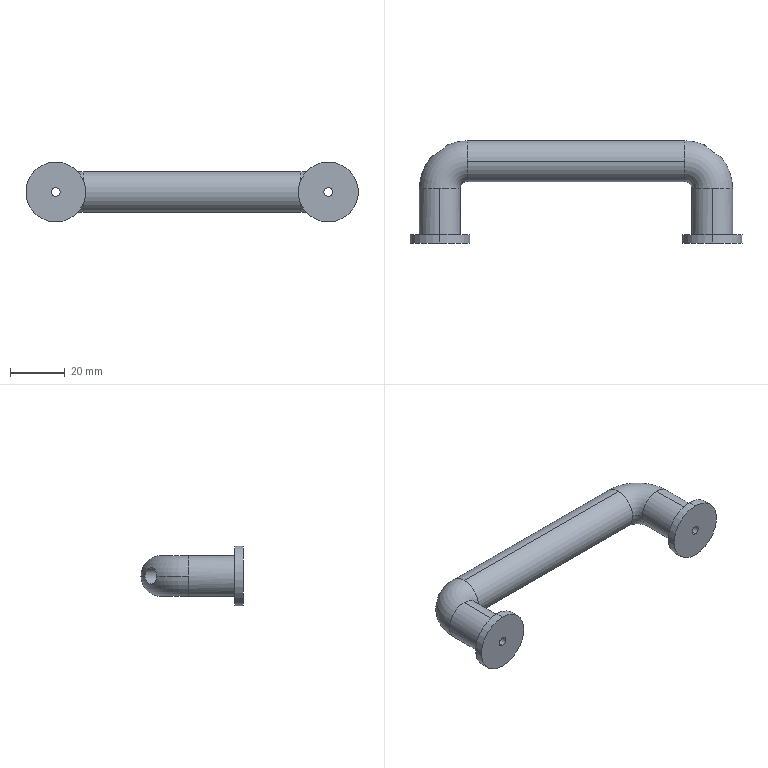Part | SolidWorks | features MirrorStock 1 | 1 solid | 28 faces | box 122 x 37.5 x 22 mm | volume 26841 mm3 | cylinder 18 | plane 6 | torus 4 | commonest cylinder face diameters 15 x6 3.3 x4 6 x4 22 x4
STEP:
#1=CARTESIAN_POINT('',(100.,20.,7.5));
#2=VERTEX_POINT('',#1);
#3=CARTESIAN_POINT('',(107.5,20.,0.));
#4=VERTEX_POINT('',#3);
#5=CARTESIAN_POINT('',(100.,20.,0.));
#6=DIRECTION('',(0.,1.,0.));
#7=DIRECTION('',(0.,0.,-1.));
#8=AXIS2_PLACEMENT_3D('',#5,#6,#7);
#9=CIRCLE('',#8,7.5);
#10=EDGE_CURVE('',#2,#4,#9,.T.);
#11=ORIENTED_EDGE('',*,*,#10,.T.);
#12=CARTESIAN_POINT('',(103.,31.715,0.));
#13=VERTEX_POINT('',#12);
#14=CARTESIAN_POINT('',(90.,20.,0.));
#15=DIRECTION('',(0.,0.,1.));
#16=DIRECTION('',(1.,0.,0.));
#17=AXIS2_PLACEMENT_3D('',#14,#15,#16);
#18=CIRCLE('',#17,17.5);
#19=EDGE_CURVE('',#4,#13,#18,.T.);
#20=ORIENTED_EDGE('',*,*,#19,.T.);
#21=CARTESIAN_POINT('',(100.,33.591,3.));
#22=VERTEX_POINT('',#21);
#23=CARTESIAN_POINT('',(103.,31.715,0.));
#24=CARTESIAN_POINT('',(103.,31.715,0.2156));
#25=CARTESIAN_POINT('',(102.976,31.727,0.4332));
#26=CARTESIAN_POINT('',(102.885,31.775,0.8502));
#27=CARTESIAN_POINT('',(102.816,31.81,1.055));
#28=CARTESIAN_POINT('',(102.64,31.904,1.44));
#29=CARTESIAN_POINT('',(102.535,31.961,1.618));
#30=CARTESIAN_POINT('',(102.293,32.095,1.945));
#31=CARTESIAN_POINT('',(102.156,32.174,2.096));
#32=CARTESIAN_POINT('',(101.863,32.345,2.359));
#33=CARTESIAN_POINT('',(101.708,32.439,2.474));
#34=CARTESIAN_POINT('',(101.381,32.642,2.67));
#35=CARTESIAN_POINT('',(101.212,32.75,2.75));
#36=CARTESIAN_POINT('',(100.7,33.089,2.94));
#37=CARTESIAN_POINT('',(100.345,33.338,3.));
#38=CARTESIAN_POINT('',(100.,33.591,3.));
#39=B_SPLINE_CURVE_WITH_KNOTS('',3,(#23,#24,#25,#26,#27,#28,#29,#30,#31,#32,#33,#34,#35,#36,#37,#38),.UNSPECIFIED.,.F.,.F.,(4,2,2,2,2,2,2,4),(0.01975,0.02039,0.02104,0.02168,0.02232,0.02296,0.0236,0.02488),.UNSPECIFIED.);
#40=EDGE_CURVE('',#13,#22,#39,.T.);
#41=ORIENTED_EDGE('',*,*,#40,.T.);
#42=CARTESIAN_POINT('',(97.,36.039,0.));
#43=VERTEX_POINT('',#42);
#44=CARTESIAN_POINT('',(100.,33.591,3.));
#45=CARTESIAN_POINT('',(99.638,33.857,3.));
#46=CARTESIAN_POINT('',(99.28,34.135,2.934));
#47=CARTESIAN_POINT('',(98.777,34.537,2.745));
#48=CARTESIAN_POINT('',(98.614,34.67,2.667));
#49=CARTESIAN_POINT('',(98.297,34.931,2.477));
#50=CARTESIAN_POINT('',(98.146,35.057,2.366));
#51=CARTESIAN_POINT('',(97.721,35.415,1.987));
#52=CARTESIAN_POINT('',(97.469,35.632,1.665));
#53=CARTESIAN_POINT('',(97.198,35.867,1.092));
#54=CARTESIAN_POINT('',(97.125,35.93,0.8836));
#55=CARTESIAN_POINT('',(97.026,36.016,0.4531));
#56=CARTESIAN_POINT('',(97.,36.039,0.2248));
#57=CARTESIAN_POINT('',(97.,36.039,0.));
#58=B_SPLINE_CURVE_WITH_KNOTS('',3,(#44,#45,#46,#47,#48,#49,#50,#51,#52,#53,#54,#55,#56,#57),.UNSPECIFIED.,.F.,.F.,(4,2,2,2,2,2,4),(0.003861,0.005206,0.005878,0.00655,0.007895,0.008567,0.009239),.UNSPECIFIED.);
#59=EDGE_CURVE('',#22,#43,#58,.T.);
#60=ORIENTED_EDGE('',*,*,#59,.T.);
#61=CARTESIAN_POINT('',(90.,37.5,0.));
#62=VERTEX_POINT('',#61);
#63=CARTESIAN_POINT('',(90.,20.,0.));
#64=DIRECTION('',(0.,0.,1.));
#65=DIRECTION('',(1.,0.,0.));
#66=AXIS2_PLACEMENT_3D('',#63,#64,#65);
#67=CIRCLE('',#66,17.5);
#68=EDGE_CURVE('',#43,#62,#67,.T.);
#69=ORIENTED_EDGE('',*,*,#68,.T.);
#70=CARTESIAN_POINT('',(90.,30.,7.5));
#71=VERTEX_POINT('',#70);
#72=CARTESIAN_POINT('',(90.,30.,0.));
#73=DIRECTION('',(-1.,0.,0.));
#74=DIRECTION('',(0.,0.,-1.));
#75=AXIS2_PLACEMENT_3D('',#72,#73,#74);
#76=CIRCLE('',#75,7.5);
#77=EDGE_CURVE('',#71,#62,#76,.T.);
#78=ORIENTED_EDGE('',*,*,#77,.F.);
#79=CARTESIAN_POINT('',(90.,22.5,0.));
#80=VERTEX_POINT('',#79);
#81=CARTESIAN_POINT('',(90.,30.,0.));
#82=DIRECTION('',(-1.,0.,0.));
#83=DIRECTION('',(0.,0.,-1.));
#84=AXIS2_PLACEMENT_3D('',#81,#82,#83);
#85=CIRCLE('',#84,7.5);
#86=EDGE_CURVE('',#80,#71,#85,.T.);
#87=ORIENTED_EDGE('',*,*,#86,.F.);
#88=CARTESIAN_POINT('',(92.5,20.,0.));
#89=VERTEX_POINT('',#88);
#90=CARTESIAN_POINT('',(90.,20.,0.));
#91=DIRECTION('',(0.,0.,1.));
#92=DIRECTION('',(1.,0.,0.));
#93=AXIS2_PLACEMENT_3D('',#90,#91,#92);
#94=CIRCLE('',#93,2.5);
#95=EDGE_CURVE('',#89,#80,#94,.T.);
#96=ORIENTED_EDGE('',*,*,#95,.F.);
#97=CARTESIAN_POINT('',(100.,20.,0.));
#98=DIRECTION('',(0.,1.,0.));
#99=DIRECTION('',(0.,0.,-1.));
#100=AXIS2_PLACEMENT_3D('',#97,#98,#99);
#101=CIRCLE('',#100,7.5);
#102=EDGE_CURVE('',#89,#2,#101,.T.);
#103=ORIENTED_EDGE('',*,*,#102,.T.);
#104=EDGE_LOOP('',(#11,#20,#41,#60,#69,#78,#87,#96,#103));
#105=FACE_OUTER_BOUND('',#104,.T.);
#106=CARTESIAN_POINT('',(90.,20.,0.));
#107=DIRECTION('',(0.,0.,1.));
#108=DIRECTION('',(-1.,0.,0.));
#109=AXIS2_PLACEMENT_3D('',#106,#107,#108);
#110=TOROIDAL_SURFACE('',#109,10.,7.5);
#111=ADVANCED_FACE('',(#105),#110,.T.);
#112=CARTESIAN_POINT('',(10.,30.,7.5));
#113=VERTEX_POINT('',#112);
#114=CARTESIAN_POINT('',(10.,37.5,0.));
#115=VERTEX_POINT('',#114);
#116=CARTESIAN_POINT('',(10.,30.,0.));
#117=DIRECTION('',(-1.,0.,0.));
#118=DIRECTION('',(0.,0.,-1.));
#119=AXIS2_PLACEMENT_3D('',#116,#117,#118);
#120=CIRCLE('',#119,7.5);
#121=EDGE_CURVE('',#113,#115,#120,.T.);
#122=ORIENTED_EDGE('',*,*,#121,.T.);
#123=CARTESIAN_POINT('',(3.,36.039,0.));
#124=VERTEX_POINT('',#123);
#125=CARTESIAN_POINT('',(10.,20.,0.));
#126=DIRECTION('',(0.,0.,1.));
#127=DIRECTION('',(1.,0.,0.));
#128=AXIS2_PLACEMENT_3D('',#125,#126,#127);
#129=CIRCLE('',#128,17.5);
#130=EDGE_CURVE('',#115,#124,#129,.T.);
#131=ORIENTED_EDGE('',*,*,#130,.T.);
#132=CARTESIAN_POINT('',(0.,33.591,3.));
#133=VERTEX_POINT('',#132);
#134=CARTESIAN_POINT('',(3.,36.039,0.));
#135=CARTESIAN_POINT('',(3.,36.039,0.2248));
#136=CARTESIAN_POINT('',(2.974,36.017,0.4506));
#137=CARTESIAN_POINT('',(2.876,35.931,0.8835));
#138=CARTESIAN_POINT('',(2.804,35.868,1.089));
#139=CARTESIAN_POINT('',(2.622,35.71,1.474));
#140=CARTESIAN_POINT('',(2.514,35.618,1.649));
#141=CARTESIAN_POINT('',(2.272,35.41,1.97));
#142=CARTESIAN_POINT('',(2.138,35.296,2.113));
#143=CARTESIAN_POINT('',(1.713,34.938,2.492));
#144=CARTESIAN_POINT('',(1.392,34.672,2.682));
#145=CARTESIAN_POINT('',(0.7188,34.134,2.935));
#146=CARTESIAN_POINT('',(0.36,33.856,3.));
#147=CARTESIAN_POINT('',(0.,33.591,3.));
#148=B_SPLINE_CURVE_WITH_KNOTS('',3,(#134,#135,#136,#137,#138,#139,#140,#141,#142,#143,#144,#145,#146,#147),.UNSPECIFIED.,.F.,.F.,(4,2,2,2,2,2,4),(0.01181,0.01248,0.01315,0.01382,0.0145,0.01584,0.01719),.UNSPECIFIED.);
#149=EDGE_CURVE('',#124,#133,#148,.T.);
#150=ORIENTED_EDGE('',*,*,#149,.T.);
#151=CARTESIAN_POINT('',(-3.,31.715,0.));
#152=VERTEX_POINT('',#151);
#153=CARTESIAN_POINT('',(0.,33.591,3.));
#154=CARTESIAN_POINT('',(-0.1721,33.465,3.));
#155=CARTESIAN_POINT('',(-0.3454,33.34,2.985));
#156=CARTESIAN_POINT('',(-0.6945,33.096,2.924));
#157=CARTESIAN_POINT('',(-0.8706,32.976,2.877));
#158=CARTESIAN_POINT('',(-1.213,32.75,2.75));
#159=CARTESIAN_POINT('',(-1.38,32.643,2.67));
#160=CARTESIAN_POINT('',(-1.707,32.44,2.475));
#161=CARTESIAN_POINT('',(-1.865,32.344,2.358));
#162=CARTESIAN_POINT('',(-2.156,32.174,2.096));
#163=CARTESIAN_POINT('',(-2.29,32.097,1.949));
#164=CARTESIAN_POINT('',(-2.534,31.962,1.619));
#165=CARTESIAN_POINT('',(-2.642,31.903,1.437));
#166=CARTESIAN_POINT('',(-2.818,31.809,1.05));
#167=CARTESIAN_POINT('',(-2.885,31.775,0.8496));
#168=CARTESIAN_POINT('',(-2.976,31.727,0.4323));
#169=CARTESIAN_POINT('',(-3.,31.715,0.2144));
#170=CARTESIAN_POINT('',(-3.,31.715,0.));
#171=B_SPLINE_CURVE_WITH_KNOTS('',3,(#153,#154,#155,#156,#157,#158,#159,#160,#161,#162,#163,#164,#165,#166,#167,#168,#169,#170),.UNSPECIFIED.,.F.,.F.,(4,2,2,2,2,2,2,2,4),(0.01719,0.01783,0.01847,0.01912,0.01976,0.0204,0.02105,0.02169,0.02233),.UNSPECIFIED.);
#172=EDGE_CURVE('',#133,#152,#171,.T.);
#173=ORIENTED_EDGE('',*,*,#172,.T.);
#174=CARTESIAN_POINT('',(-7.5,20.,0.));
#175=VERTEX_POINT('',#174);
#176=CARTESIAN_POINT('',(10.,20.,0.));
#177=DIRECTION('',(0.,0.,1.));
#178=DIRECTION('',(1.,0.,0.));
#179=AXIS2_PLACEMENT_3D('',#176,#177,#178);
#180=CIRCLE('',#179,17.5);
#181=EDGE_CURVE('',#152,#175,#180,.T.);
#182=ORIENTED_EDGE('',*,*,#181,.T.);
#183=CARTESIAN_POINT('',(0.,20.,7.5));
#184=VERTEX_POINT('',#183);
#185=CARTESIAN_POINT('',(0.,20.,0.));
#186=DIRECTION('',(0.,-1.,0.));
#187=DIRECTION('',(0.,0.,-1.));
#188=AXIS2_PLACEMENT_3D('',#185,#186,#187);
#189=CIRCLE('',#188,7.5);
#190=EDGE_CURVE('',#184,#175,#189,.T.);
#191=ORIENTED_EDGE('',*,*,#190,.F.);
#192=CARTESIAN_POINT('',(7.5,20.,0.));
#193=VERTEX_POINT('',#192);
#194=CARTESIAN_POINT('',(0.,20.,0.));
#195=DIRECTION('',(0.,-1.,0.));
#196=DIRECTION('',(0.,0.,-1.));
#197=AXIS2_PLACEMENT_3D('',#194,#195,#196);
#198=CIRCLE('',#197,7.5);
#199=EDGE_CURVE('',#193,#184,#198,.T.);
#200=ORIENTED_EDGE('',*,*,#199,.F.);
#201=CARTESIAN_POINT('',(10.,22.5,0.));
#202=VERTEX_POINT('',#201);
#203=CARTESIAN_POINT('',(10.,20.,0.));
#204=DIRECTION('',(0.,0.,1.));
#205=DIRECTION('',(1.,0.,0.));
#206=AXIS2_PLACEMENT_3D('',#203,#204,#205);
#207=CIRCLE('',#206,2.5);
#208=EDGE_CURVE('',#202,#193,#207,.T.);
#209=ORIENTED_EDGE('',*,*,#208,.F.);
#210=CARTESIAN_POINT('',(10.,30.,0.));
#211=DIRECTION('',(-1.,0.,0.));
#212=DIRECTION('',(0.,0.,-1.));
#213=AXIS2_PLACEMENT_3D('',#210,#211,#212);
#214=CIRCLE('',#213,7.5);
#215=EDGE_CURVE('',#202,#113,#214,.T.);
#216=ORIENTED_EDGE('',*,*,#215,.T.);
#217=EDGE_LOOP('',(#122,#131,#150,#173,#182,#191,#200,#209,#216));
#218=FACE_OUTER_BOUND('',#217,.T.);
#219=CARTESIAN_POINT('',(10.,20.,0.));
#220=DIRECTION('',(0.,0.,1.));
#221=DIRECTION('',(-1.,0.,0.));
#222=AXIS2_PLACEMENT_3D('',#219,#220,#221);
#223=TOROIDAL_SURFACE('',#222,10.,7.5);
#224=ADVANCED_FACE('',(#218),#223,.T.);
#225=CARTESIAN_POINT('',(100.,33.591,-3.));
#226=VERTEX_POINT('',#225);
#227=CARTESIAN_POINT('',(100.,33.591,-3.));
#228=CARTESIAN_POINT('',(100.172,33.465,-3.));
#229=CARTESIAN_POINT('',(100.346,33.34,-2.985));
#230=CARTESIAN_POINT('',(100.696,33.095,-2.924));
#231=CARTESIAN_POINT('',(100.872,32.976,-2.876));
#232=CARTESIAN_POINT('',(101.214,32.749,-2.75));
#233=CARTESIAN_POINT('',(101.382,32.642,-2.67));
#234=CARTESIAN_POINT('',(101.709,32.438,-2.473));
#235=CARTESIAN_POINT('',(101.866,32.343,-2.357));
#236=CARTESIAN_POINT('',(102.157,32.173,-2.094));
#237=CARTESIAN_POINT('',(102.292,32.096,-1.947));
#238=CARTESIAN_POINT('',(102.536,31.96,-1.616));
#239=CARTESIAN_POINT('',(102.643,31.903,-1.435));
#240=CARTESIAN_POINT('',(102.816,31.81,-1.054));
#241=CARTESIAN_POINT('',(102.885,31.775,-0.8506));
#242=CARTESIAN_POINT('',(102.977,31.727,-0.4294));
#243=CARTESIAN_POINT('',(103.,31.715,-0.2161));
#244=CARTESIAN_POINT('',(103.,31.715,0.));
#245=B_SPLINE_CURVE_WITH_KNOTS('',3,(#227,#228,#229,#230,#231,#232,#233,#234,#235,#236,#237,#238,#239,#240,#241,#242,#243,#244),.UNSPECIFIED.,.F.,.F.,(4,2,2,2,2,2,2,2,4),(0.01461,0.01525,0.0159,0.01654,0.01718,0.01783,0.01847,0.01911,0.01975),.UNSPECIFIED.);
#246=EDGE_CURVE('',#226,#13,#245,.T.);
#247=ORIENTED_EDGE('',*,*,#246,.F.);
#248=CARTESIAN_POINT('',(100.,20.,-3.));
#249=VERTEX_POINT('',#248);
#250=CARTESIAN_POINT('',(100.,71.,-3.));
#251=DIRECTION('',(0.,-1.,0.));
#252=VECTOR('',#251,1000.);
#253=LINE('',#250,#252);
#254=EDGE_CURVE('',#226,#249,#253,.T.);
#255=ORIENTED_EDGE('',*,*,#254,.T.);
#256=CARTESIAN_POINT('',(100.,20.,3.));
#257=VERTEX_POINT('',#256);
#258=CARTESIAN_POINT('',(100.,20.,0.));
#259=DIRECTION('',(0.,1.,0.));
#260=DIRECTION('',(0.,0.,1.));
#261=AXIS2_PLACEMENT_3D('',#258,#259,#260);
#262=CIRCLE('',#261,3.);
#263=EDGE_CURVE('',#257,#249,#262,.T.);
#264=ORIENTED_EDGE('',*,*,#263,.F.);
#265=CARTESIAN_POINT('',(100.,71.,3.));
#266=DIRECTION('',(0.,-1.,0.));
#267=VECTOR('',#266,1000.);
#268=LINE('',#265,#267);
#269=EDGE_CURVE('',#22,#257,#268,.T.);
#270=ORIENTED_EDGE('',*,*,#269,.F.);
#271=ORIENTED_EDGE('',*,*,#40,.F.);
#272=EDGE_LOOP('',(#247,#255,#264,#270,#271));
#273=FACE_OUTER_BOUND('',#272,.T.);
#274=CARTESIAN_POINT('',(100.,71.,0.));
#275=DIRECTION('',(0.,-1.,0.));
#276=DIRECTION('',(0.,0.,1.));
#277=AXIS2_PLACEMENT_3D('',#274,#275,#276);
#278=CYLINDRICAL_SURFACE('',#277,3.);
#279=ADVANCED_FACE('',(#273),#278,.F.);
#280=CARTESIAN_POINT('',(0.,33.591,-3.));
#281=VERTEX_POINT('',#280);
#282=CARTESIAN_POINT('',(0.,33.591,-3.));
#283=CARTESIAN_POINT('',(0.3615,33.857,-3.));
#284=CARTESIAN_POINT('',(0.7202,34.135,-2.934));
#285=CARTESIAN_POINT('',(1.223,34.537,-2.745));
#286=CARTESIAN_POINT('',(1.386,34.67,-2.667));
#287=CARTESIAN_POINT('',(1.702,34.93,-2.477));
#288=CARTESIAN_POINT('',(1.854,35.057,-2.366));
#289=CARTESIAN_POINT('',(2.138,35.296,-2.113));
#290=CARTESIAN_POINT('',(2.27,35.409,-1.971));
#291=CARTESIAN_POINT('',(2.514,35.618,-1.649));
#292=CARTESIAN_POINT('',(2.621,35.71,-1.474));
#293=CARTESIAN_POINT('',(2.802,35.867,-1.092));
#294=CARTESIAN_POINT('',(2.875,35.93,-0.8837));
#295=CARTESIAN_POINT('',(2.974,36.016,-0.4532));
#296=CARTESIAN_POINT('',(3.,36.039,-0.225));
#297=CARTESIAN_POINT('',(3.,36.039,0.));
#298=B_SPLINE_CURVE_WITH_KNOTS('',3,(#282,#283,#284,#285,#286,#287,#288,#289,#290,#291,#292,#293,#294,#295,#296,#297),.UNSPECIFIED.,.F.,.F.,(4,2,2,2,2,2,2,4),(0.00642,0.007767,0.00844,0.009113,0.009787,0.01046,0.01113,0.01181),.UNSPECIFIED.);
#299=EDGE_CURVE('',#281,#124,#298,.T.);
#300=ORIENTED_EDGE('',*,*,#299,.F.);
#301=CARTESIAN_POINT('',(0.,20.,-3.));
#302=VERTEX_POINT('',#301);
#303=CARTESIAN_POINT('',(0.,71.,-3.));
#304=DIRECTION('',(0.,-1.,0.));
#305=VECTOR('',#304,1000.);
#306=LINE('',#303,#305);
#307=EDGE_CURVE('',#281,#302,#306,.T.);
#308=ORIENTED_EDGE('',*,*,#307,.T.);
#309=CARTESIAN_POINT('',(0.,20.,3.));
#310=VERTEX_POINT('',#309);
#311=CARTESIAN_POINT('',(0.,20.,0.));
#312=DIRECTION('',(0.,1.,0.));
#313=DIRECTION('',(0.,0.,1.));
#314=AXIS2_PLACEMENT_3D('',#311,#312,#313);
#315=CIRCLE('',#314,3.);
#316=EDGE_CURVE('',#310,#302,#315,.T.);
#317=ORIENTED_EDGE('',*,*,#316,.F.);
#318=CARTESIAN_POINT('',(0.,71.,3.));
#319=DIRECTION('',(0.,-1.,0.));
#320=VECTOR('',#319,1000.);
#321=LINE('',#318,#320);
#322=EDGE_CURVE('',#133,#310,#321,.T.);
#323=ORIENTED_EDGE('',*,*,#322,.F.);
#324=ORIENTED_EDGE('',*,*,#149,.F.);
#325=EDGE_LOOP('',(#300,#308,#317,#323,#324));
#326=FACE_OUTER_BOUND('',#325,.T.);
#327=CARTESIAN_POINT('',(0.,71.,0.));
#328=DIRECTION('',(0.,-1.,0.));
#329=DIRECTION('',(0.,0.,1.));
#330=AXIS2_PLACEMENT_3D('',#327,#328,#329);
#331=CYLINDRICAL_SURFACE('',#330,3.);
#332=ADVANCED_FACE('',(#326),#331,.F.);
#333=CARTESIAN_POINT('',(0.,20.,-1.65));
#334=VERTEX_POINT('',#333);
#335=CARTESIAN_POINT('',(0.,20.,1.65));
#336=VERTEX_POINT('',#335);
#337=CARTESIAN_POINT('',(0.,20.,0.));
#338=DIRECTION('',(0.,-1.,0.));
#339=DIRECTION('',(0.,0.,1.));
#340=AXIS2_PLACEMENT_3D('',#337,#338,#339);
#341=CIRCLE('',#340,1.65);
#342=EDGE_CURVE('',#334,#336,#341,.T.);
#343=ORIENTED_EDGE('',*,*,#342,.F.);
#344=CARTESIAN_POINT('',(0.,0.,-1.65));
#345=VERTEX_POINT('',#344);
#346=CARTESIAN_POINT('',(0.,51.,-1.65));
#347=DIRECTION('',(0.,-1.,0.));
#348=VECTOR('',#347,1000.);
#349=LINE('',#346,#348);
#350=EDGE_CURVE('',#334,#345,#349,.T.);
#351=ORIENTED_EDGE('',*,*,#350,.T.);
#352=CARTESIAN_POINT('',(0.,0.,1.65));
#353=VERTEX_POINT('',#352);
#354=CARTESIAN_POINT('',(0.,0.,0.));
#355=DIRECTION('',(0.,1.,0.));
#356=DIRECTION('',(0.,0.,1.));
#357=AXIS2_PLACEMENT_3D('',#354,#355,#356);
#358=CIRCLE('',#357,1.65);
#359=EDGE_CURVE('',#353,#345,#358,.T.);
#360=ORIENTED_EDGE('',*,*,#359,.F.);
#361=CARTESIAN_POINT('',(0.,51.,1.65));
#362=DIRECTION('',(0.,-1.,0.));
#363=VECTOR('',#362,1000.);
#364=LINE('',#361,#363);
#365=EDGE_CURVE('',#336,#353,#364,.T.);
#366=ORIENTED_EDGE('',*,*,#365,.F.);
#367=EDGE_LOOP('',(#343,#351,#360,#366));
#368=FACE_OUTER_BOUND('',#367,.T.);
#369=CARTESIAN_POINT('',(0.,51.,0.));
#370=DIRECTION('',(0.,-1.,0.));
#371=DIRECTION('',(0.,0.,1.));
#372=AXIS2_PLACEMENT_3D('',#369,#370,#371);
#373=CYLINDRICAL_SURFACE('',#372,1.65);
#374=ADVANCED_FACE('',(#368),#373,.F.);
#375=CARTESIAN_POINT('',(100.,20.,-1.65));
#376=VERTEX_POINT('',#375);
#377=CARTESIAN_POINT('',(100.,20.,1.65));
#378=VERTEX_POINT('',#377);
#379=CARTESIAN_POINT('',(100.,20.,0.));
#380=DIRECTION('',(0.,-1.,0.));
#381=DIRECTION('',(0.,0.,1.));
#382=AXIS2_PLACEMENT_3D('',#379,#380,#381);
#383=CIRCLE('',#382,1.65);
#384=EDGE_CURVE('',#376,#378,#383,.T.);
#385=ORIENTED_EDGE('',*,*,#384,.F.);
#386=CARTESIAN_POINT('',(100.,0.,-1.65));
#387=VERTEX_POINT('',#386);
#388=CARTESIAN_POINT('',(100.,51.,-1.65));
#389=DIRECTION('',(0.,-1.,0.));
#390=VECTOR('',#389,1000.);
#391=LINE('',#388,#390);
#392=EDGE_CURVE('',#376,#387,#391,.T.);
#393=ORIENTED_EDGE('',*,*,#392,.T.);
#394=CARTESIAN_POINT('',(100.,0.,1.65));
#395=VERTEX_POINT('',#394);
#396=CARTESIAN_POINT('',(100.,0.,0.));
#397=DIRECTION('',(0.,1.,0.));
#398=DIRECTION('',(0.,0.,1.));
#399=AXIS2_PLACEMENT_3D('',#396,#397,#398);
#400=CIRCLE('',#399,1.65);
#401=EDGE_CURVE('',#395,#387,#400,.T.);
#402=ORIENTED_EDGE('',*,*,#401,.F.);
#403=CARTESIAN_POINT('',(100.,51.,1.65));
#404=DIRECTION('',(0.,-1.,0.));
#405=VECTOR('',#404,1000.);
#406=LINE('',#403,#405);
#407=EDGE_CURVE('',#378,#395,#406,.T.);
#408=ORIENTED_EDGE('',*,*,#407,.F.);
#409=EDGE_LOOP('',(#385,#393,#402,#408));
#410=FACE_OUTER_BOUND('',#409,.T.);
#411=CARTESIAN_POINT('',(100.,51.,0.));
#412=DIRECTION('',(0.,-1.,0.));
#413=DIRECTION('',(0.,0.,1.));
#414=AXIS2_PLACEMENT_3D('',#411,#412,#413);
#415=CYLINDRICAL_SURFACE('',#414,1.65);
#416=ADVANCED_FACE('',(#410),#415,.F.);
#417=CARTESIAN_POINT('',(100.,3.,-11.));
#418=VERTEX_POINT('',#417);
#419=CARTESIAN_POINT('',(100.,3.,11.));
#420=VERTEX_POINT('',#419);
#421=CARTESIAN_POINT('',(100.,3.,0.));
#422=DIRECTION('',(0.,1.,0.));
#423=DIRECTION('',(0.,0.,1.));
#424=AXIS2_PLACEMENT_3D('',#421,#422,#423);
#425=CIRCLE('',#424,11.);
#426=EDGE_CURVE('',#418,#420,#425,.T.);
#427=ORIENTED_EDGE('',*,*,#426,.F.);
#428=CARTESIAN_POINT('',(100.,0.,-11.));
#429=VERTEX_POINT('',#428);
#430=CARTESIAN_POINT('',(100.,3.,-11.));
#431=DIRECTION('',(0.,-1.,0.));
#432=VECTOR('',#431,1000.);
#433=LINE('',#430,#432);
#434=EDGE_CURVE('',#418,#429,#433,.T.);
#435=ORIENTED_EDGE('',*,*,#434,.T.);
#436=CARTESIAN_POINT('',(100.,0.,11.));
#437=VERTEX_POINT('',#436);
#438=CARTESIAN_POINT('',(100.,0.,0.));
#439=DIRECTION('',(0.,1.,0.));
#440=DIRECTION('',(0.,0.,1.));
#441=AXIS2_PLACEMENT_3D('',#438,#439,#440);
#442=CIRCLE('',#441,11.);
#443=EDGE_CURVE('',#429,#437,#442,.T.);
#444=ORIENTED_EDGE('',*,*,#443,.T.);
#445=CARTESIAN_POINT('',(100.,3.,11.));
#446=DIRECTION('',(0.,-1.,0.));
#447=VECTOR('',#446,1000.);
#448=LINE('',#445,#447);
#449=EDGE_CURVE('',#420,#437,#448,.T.);
#450=ORIENTED_EDGE('',*,*,#449,.F.);
#451=EDGE_LOOP('',(#427,#435,#444,#450));
#452=FACE_OUTER_BOUND('',#451,.T.);
#453=CARTESIAN_POINT('',(100.,3.,0.));
#454=DIRECTION('',(0.,-1.,0.));
#455=DIRECTION('',(0.,0.,1.));
#456=AXIS2_PLACEMENT_3D('',#453,#454,#455);
#457=CYLINDRICAL_SURFACE('',#456,11.);
#458=ADVANCED_FACE('',(#452),#457,.T.);
#459=CARTESIAN_POINT('',(0.,3.,-11.));
#460=VERTEX_POINT('',#459);
#461=CARTESIAN_POINT('',(0.,3.,11.));
#462=VERTEX_POINT('',#461);
#463=CARTESIAN_POINT('',(0.,3.,0.));
#464=DIRECTION('',(0.,1.,0.));
#465=DIRECTION('',(0.,0.,1.));
#466=AXIS2_PLACEMENT_3D('',#463,#464,#465);
#467=CIRCLE('',#466,11.);
#468=EDGE_CURVE('',#460,#462,#467,.T.);
#469=ORIENTED_EDGE('',*,*,#468,.F.);
#470=CARTESIAN_POINT('',(0.,0.,-11.));
#471=VERTEX_POINT('',#470);
#472=CARTESIAN_POINT('',(0.,3.,-11.));
#473=DIRECTION('',(0.,-1.,0.));
#474=VECTOR('',#473,1000.);
#475=LINE('',#472,#474);
#476=EDGE_CURVE('',#460,#471,#475,.T.);
#477=ORIENTED_EDGE('',*,*,#476,.T.);
#478=CARTESIAN_POINT('',(0.,0.,11.));
#479=VERTEX_POINT('',#478);
#480=CARTESIAN_POINT('',(0.,0.,0.));
#481=DIRECTION('',(0.,1.,0.));
#482=DIRECTION('',(0.,0.,1.));
#483=AXIS2_PLACEMENT_3D('',#480,#481,#482);
#484=CIRCLE('',#483,11.);
#485=EDGE_CURVE('',#471,#479,#484,.T.);
#486=ORIENTED_EDGE('',*,*,#485,.T.);
#487=CARTESIAN_POINT('',(0.,3.,11.));
#488=DIRECTION('',(0.,-1.,0.));
#489=VECTOR('',#488,1000.);
#490=LINE('',#487,#489);
#491=EDGE_CURVE('',#462,#479,#490,.T.);
#492=ORIENTED_EDGE('',*,*,#491,.F.);
#493=EDGE_LOOP('',(#469,#477,#486,#492));
#494=FACE_OUTER_BOUND('',#493,.T.);
#495=CARTESIAN_POINT('',(0.,3.,0.));
#496=DIRECTION('',(0.,-1.,0.));
#497=DIRECTION('',(0.,0.,1.));
#498=AXIS2_PLACEMENT_3D('',#495,#496,#497);
#499=CYLINDRICAL_SURFACE('',#498,11.);
#500=ADVANCED_FACE('',(#494),#499,.T.);
#501=CARTESIAN_POINT('',(10.,30.,-7.5));
#502=VERTEX_POINT('',#501);
#503=CARTESIAN_POINT('',(10.,30.,0.));
#504=DIRECTION('',(-1.,0.,0.));
#505=DIRECTION('',(0.,0.,-1.));
#506=AXIS2_PLACEMENT_3D('',#503,#504,#505);
#507=CIRCLE('',#506,7.5);
#508=EDGE_CURVE('',#502,#202,#507,.T.);
#509=ORIENTED_EDGE('',*,*,#508,.F.);
#510=CARTESIAN_POINT('',(90.,30.,-7.5));
#511=VERTEX_POINT('',#510);
#512=CARTESIAN_POINT('',(10.,30.,-7.5));
#513=DIRECTION('',(1.,0.,0.));
#514=VECTOR('',#513,1000.);
#515=LINE('',#512,#514);
#516=EDGE_CURVE('',#502,#511,#515,.T.);
#517=ORIENTED_EDGE('',*,*,#516,.T.);
#518=CARTESIAN_POINT('',(90.,30.,0.));
#519=DIRECTION('',(-1.,0.,0.));
#520=DIRECTION('',(0.,0.,-1.));
#521=AXIS2_PLACEMENT_3D('',#518,#519,#520);
#522=CIRCLE('',#521,7.5);
#523=EDGE_CURVE('',#511,#80,#522,.T.);
#524=ORIENTED_EDGE('',*,*,#523,.T.);
#525=ORIENTED_EDGE('',*,*,#86,.T.);
#526=CARTESIAN_POINT('',(10.,30.,7.5));
#527=DIRECTION('',(1.,0.,0.));
#528=VECTOR('',#527,1000.);
#529=LINE('',#526,#528);
#530=EDGE_CURVE('',#113,#71,#529,.T.);
#531=ORIENTED_EDGE('',*,*,#530,.F.);
#532=ORIENTED_EDGE('',*,*,#215,.F.);
#533=EDGE_LOOP('',(#509,#517,#524,#525,#531,#532));
#534=FACE_OUTER_BOUND('',#533,.T.);
#535=CARTESIAN_POINT('',(10.,30.,0.));
#536=DIRECTION('',(1.,0.,0.));
#537=DIRECTION('',(0.,0.,1.));
#538=AXIS2_PLACEMENT_3D('',#535,#536,#537);
#539=CYLINDRICAL_SURFACE('',#538,7.5);
#540=ADVANCED_FACE('',(#534),#539,.T.);
#541=CARTESIAN_POINT('',(0.,3.,7.5));
#542=VERTEX_POINT('',#541);
#543=CARTESIAN_POINT('',(0.,3.,-7.5));
#544=VERTEX_POINT('',#543);
#545=CARTESIAN_POINT('',(0.,3.,0.));
#546=DIRECTION('',(0.,-1.,0.));
#547=DIRECTION('',(0.,0.,1.));
#548=AXIS2_PLACEMENT_3D('',#545,#546,#547);
#549=CIRCLE('',#548,7.5);
#550=EDGE_CURVE('',#542,#544,#549,.T.);
#551=ORIENTED_EDGE('',*,*,#550,.F.);
#552=CARTESIAN_POINT('',(0.,0.,7.5));
#553=DIRECTION('',(0.,1.,0.));
#554=VECTOR('',#553,1000.);
#555=LINE('',#552,#554);
#556=EDGE_CURVE('',#542,#184,#555,.T.);
#557=ORIENTED_EDGE('',*,*,#556,.T.);
#558=ORIENTED_EDGE('',*,*,#190,.T.);
#559=CARTESIAN_POINT('',(0.,20.,-7.5));
#560=VERTEX_POINT('',#559);
#561=CARTESIAN_POINT('',(0.,20.,0.));
#562=DIRECTION('',(0.,-1.,0.));
#563=DIRECTION('',(0.,0.,-1.));
#564=AXIS2_PLACEMENT_3D('',#561,#562,#563);
#565=CIRCLE('',#564,7.5);
#566=EDGE_CURVE('',#175,#560,#565,.T.);
#567=ORIENTED_EDGE('',*,*,#566,.T.);
#568=CARTESIAN_POINT('',(0.,0.,-7.5));
#569=DIRECTION('',(0.,1.,0.));
#570=VECTOR('',#569,1000.);
#571=LINE('',#568,#570);
#572=EDGE_CURVE('',#544,#560,#571,.T.);
#573=ORIENTED_EDGE('',*,*,#572,.F.);
#574=EDGE_LOOP('',(#551,#557,#558,#567,#573));
#575=FACE_OUTER_BOUND('',#574,.T.);
#576=CARTESIAN_POINT('',(0.,0.,0.));
#577=DIRECTION('',(0.,1.,0.));
#578=DIRECTION('',(0.,0.,-1.));
#579=AXIS2_PLACEMENT_3D('',#576,#577,#578);
#580=CYLINDRICAL_SURFACE('',#579,7.5);
#581=ADVANCED_FACE('',(#575),#580,.T.);
#582=CARTESIAN_POINT('',(100.,20.,-7.5));
#583=VERTEX_POINT('',#582);
#584=CARTESIAN_POINT('',(100.,20.,0.));
#585=DIRECTION('',(0.,1.,0.));
#586=DIRECTION('',(0.,0.,-1.));
#587=AXIS2_PLACEMENT_3D('',#584,#585,#586);
#588=CIRCLE('',#587,7.5);
#589=EDGE_CURVE('',#583,#89,#588,.T.);
#590=ORIENTED_EDGE('',*,*,#589,.F.);
#591=CARTESIAN_POINT('',(100.,3.,-7.5));
#592=VERTEX_POINT('',#591);
#593=CARTESIAN_POINT('',(100.,20.,-7.5));
#594=DIRECTION('',(0.,-1.,0.));
#595=VECTOR('',#594,1000.);
#596=LINE('',#593,#595);
#597=EDGE_CURVE('',#583,#592,#596,.T.);
#598=ORIENTED_EDGE('',*,*,#597,.T.);
#599=CARTESIAN_POINT('',(100.,3.,7.5));
#600=VERTEX_POINT('',#599);
#601=CARTESIAN_POINT('',(100.,3.,0.));
#602=DIRECTION('',(0.,-1.,0.));
#603=DIRECTION('',(0.,0.,1.));
#604=AXIS2_PLACEMENT_3D('',#601,#602,#603);
#605=CIRCLE('',#604,7.5);
#606=EDGE_CURVE('',#600,#592,#605,.T.);
#607=ORIENTED_EDGE('',*,*,#606,.F.);
#608=CARTESIAN_POINT('',(100.,20.,7.5));
#609=DIRECTION('',(0.,-1.,0.));
#610=VECTOR('',#609,1000.);
#611=LINE('',#608,#610);
#612=EDGE_CURVE('',#2,#600,#611,.T.);
#613=ORIENTED_EDGE('',*,*,#612,.F.);
#614=ORIENTED_EDGE('',*,*,#102,.F.);
#615=EDGE_LOOP('',(#590,#598,#607,#613,#614));
#616=FACE_OUTER_BOUND('',#615,.T.);
#617=CARTESIAN_POINT('',(100.,20.,0.));
#618=DIRECTION('',(0.,-1.,0.));
#619=DIRECTION('',(0.,0.,1.));
#620=AXIS2_PLACEMENT_3D('',#617,#618,#619);
#621=CYLINDRICAL_SURFACE('',#620,7.5);
#622=ADVANCED_FACE('',(#616),#621,.T.);
#623=ORIENTED_EDGE('',*,*,#597,.F.);
#624=CARTESIAN_POINT('',(100.,20.,0.));
#625=DIRECTION('',(0.,1.,0.));
#626=DIRECTION('',(0.,0.,-1.));
#627=AXIS2_PLACEMENT_3D('',#624,#625,#626);
#628=CIRCLE('',#627,7.5);
#629=EDGE_CURVE('',#4,#583,#628,.T.);
#630=ORIENTED_EDGE('',*,*,#629,.F.);
#631=ORIENTED_EDGE('',*,*,#10,.F.);
#632=ORIENTED_EDGE('',*,*,#612,.T.);
#633=CARTESIAN_POINT('',(100.,3.,0.));
#634=DIRECTION('',(0.,-1.,0.));
#635=DIRECTION('',(0.,0.,1.));
#636=AXIS2_PLACEMENT_3D('',#633,#634,#635);
#637=CIRCLE('',#636,7.5);
#638=EDGE_CURVE('',#592,#600,#637,.T.);
#639=ORIENTED_EDGE('',*,*,#638,.F.);
#640=EDGE_LOOP('',(#623,#630,#631,#632,#639));
#641=FACE_OUTER_BOUND('',#640,.T.);
#642=CARTESIAN_POINT('',(100.,20.,0.));
#643=DIRECTION('',(0.,-1.,0.));
#644=DIRECTION('',(0.,0.,1.));
#645=AXIS2_PLACEMENT_3D('',#642,#643,#644);
#646=CYLINDRICAL_SURFACE('',#645,7.5);
#647=ADVANCED_FACE('',(#641),#646,.T.);
#648=ORIENTED_EDGE('',*,*,#556,.F.);
#649=CARTESIAN_POINT('',(0.,3.,0.));
#650=DIRECTION('',(0.,-1.,0.));
#651=DIRECTION('',(0.,0.,1.));
#652=AXIS2_PLACEMENT_3D('',#649,#650,#651);
#653=CIRCLE('',#652,7.5);
#654=EDGE_CURVE('',#544,#542,#653,.T.);
#655=ORIENTED_EDGE('',*,*,#654,.F.);
#656=ORIENTED_EDGE('',*,*,#572,.T.);
#657=CARTESIAN_POINT('',(0.,20.,0.));
#658=DIRECTION('',(0.,-1.,0.));
#659=DIRECTION('',(0.,0.,-1.));
#660=AXIS2_PLACEMENT_3D('',#657,#658,#659);
#661=CIRCLE('',#660,7.5);
#662=EDGE_CURVE('',#560,#193,#661,.T.);
#663=ORIENTED_EDGE('',*,*,#662,.T.);
#664=ORIENTED_EDGE('',*,*,#199,.T.);
#665=EDGE_LOOP('',(#648,#655,#656,#663,#664));
#666=FACE_OUTER_BOUND('',#665,.T.);
#667=CARTESIAN_POINT('',(0.,0.,0.));
#668=DIRECTION('',(0.,1.,0.));
#669=DIRECTION('',(0.,0.,-1.));
#670=AXIS2_PLACEMENT_3D('',#667,#668,#669);
#671=CYLINDRICAL_SURFACE('',#670,7.5);
#672=ADVANCED_FACE('',(#666),#671,.T.);
#673=ORIENTED_EDGE('',*,*,#130,.F.);
#674=CARTESIAN_POINT('',(10.,30.,0.));
#675=DIRECTION('',(-1.,0.,0.));
#676=DIRECTION('',(0.,0.,-1.));
#677=AXIS2_PLACEMENT_3D('',#674,#675,#676);
#678=CIRCLE('',#677,7.5);
#679=EDGE_CURVE('',#115,#502,#678,.T.);
#680=ORIENTED_EDGE('',*,*,#679,.T.);
#681=ORIENTED_EDGE('',*,*,#508,.T.);
#682=ORIENTED_EDGE('',*,*,#208,.T.);
#683=ORIENTED_EDGE('',*,*,#662,.F.);
#684=ORIENTED_EDGE('',*,*,#566,.F.);
#685=ORIENTED_EDGE('',*,*,#181,.F.);
#686=CARTESIAN_POINT('',(-3.,31.715,0.));
#687=CARTESIAN_POINT('',(-3.,31.715,-0.2143));
#688=CARTESIAN_POINT('',(-2.977,31.727,-0.4299));
#689=CARTESIAN_POINT('',(-2.885,31.775,-0.8497));
#690=CARTESIAN_POINT('',(-2.818,31.81,-1.05));
#691=CARTESIAN_POINT('',(-2.644,31.902,-1.434));
#692=CARTESIAN_POINT('',(-2.537,31.96,-1.615));
#693=CARTESIAN_POINT('',(-2.295,32.094,-1.943));
#694=CARTESIAN_POINT('',(-2.158,32.172,-2.094));
#695=CARTESIAN_POINT('',(-1.865,32.344,-2.358));
#696=CARTESIAN_POINT('',(-1.709,32.438,-2.473));
#697=CARTESIAN_POINT('',(-1.383,32.641,-2.669));
#698=CARTESIAN_POINT('',(-1.213,32.75,-2.75));
#699=CARTESIAN_POINT('',(-0.7004,33.089,-2.94));
#700=CARTESIAN_POINT('',(-0.3451,33.338,-3.));
#701=CARTESIAN_POINT('',(0.,33.591,-3.));
#702=B_SPLINE_CURVE_WITH_KNOTS('',3,(#686,#687,#688,#689,#690,#691,#692,#693,#694,#695,#696,#697,#698,#699,#700,#701),.UNSPECIFIED.,.F.,.F.,(4,2,2,2,2,2,2,4),(0.001277,0.00192,0.002563,0.003206,0.003848,0.004491,0.005134,0.00642),.UNSPECIFIED.);
#703=EDGE_CURVE('',#152,#281,#702,.T.);
#704=ORIENTED_EDGE('',*,*,#703,.T.);
#705=ORIENTED_EDGE('',*,*,#299,.T.);
#706=EDGE_LOOP('',(#673,#680,#681,#682,#683,#684,#685,#704,#705));
#707=FACE_OUTER_BOUND('',#706,.T.);
#708=CARTESIAN_POINT('',(10.,20.,0.));
#709=DIRECTION('',(0.,0.,1.));
#710=DIRECTION('',(-1.,0.,0.));
#711=AXIS2_PLACEMENT_3D('',#708,#709,#710);
#712=TOROIDAL_SURFACE('',#711,10.,7.5);
#713=ADVANCED_FACE('',(#707),#712,.T.);
#714=ORIENTED_EDGE('',*,*,#516,.F.);
#715=ORIENTED_EDGE('',*,*,#679,.F.);
#716=ORIENTED_EDGE('',*,*,#121,.F.);
#717=ORIENTED_EDGE('',*,*,#530,.T.);
#718=ORIENTED_EDGE('',*,*,#77,.T.);
#719=CARTESIAN_POINT('',(90.,30.,0.));
#720=DIRECTION('',(-1.,0.,0.));
#721=DIRECTION('',(0.,0.,-1.));
#722=AXIS2_PLACEMENT_3D('',#719,#720,#721);
#723=CIRCLE('',#722,7.5);
#724=EDGE_CURVE('',#62,#511,#723,.T.);
#725=ORIENTED_EDGE('',*,*,#724,.T.);
#726=EDGE_LOOP('',(#714,#715,#716,#717,#718,#725));
#727=FACE_OUTER_BOUND('',#726,.T.);
#728=CARTESIAN_POINT('',(10.,30.,0.));
#729=DIRECTION('',(1.,0.,0.));
#730=DIRECTION('',(0.,0.,1.));
#731=AXIS2_PLACEMENT_3D('',#728,#729,#730);
#732=CYLINDRICAL_SURFACE('',#731,7.5);
#733=ADVANCED_FACE('',(#727),#732,.T.);
#734=ORIENTED_EDGE('',*,*,#19,.F.);
#735=ORIENTED_EDGE('',*,*,#629,.T.);
#736=ORIENTED_EDGE('',*,*,#589,.T.);
#737=ORIENTED_EDGE('',*,*,#95,.T.);
#738=ORIENTED_EDGE('',*,*,#523,.F.);
#739=ORIENTED_EDGE('',*,*,#724,.F.);
#740=ORIENTED_EDGE('',*,*,#68,.F.);
#741=CARTESIAN_POINT('',(97.,36.039,0.));
#742=CARTESIAN_POINT('',(97.,36.039,-0.1123));
#743=CARTESIAN_POINT('',(97.006,36.034,-0.2242));
#744=CARTESIAN_POINT('',(97.031,36.012,-0.4473));
#745=CARTESIAN_POINT('',(97.05,35.995,-0.5591));
#746=CARTESIAN_POINT('',(97.124,35.931,-0.8834));
#747=CARTESIAN_POINT('',(97.197,35.868,-1.089));
#748=CARTESIAN_POINT('',(97.469,35.632,-1.666));
#749=CARTESIAN_POINT('',(97.721,35.415,-1.987));
#750=CARTESIAN_POINT('',(98.287,34.938,-2.492));
#751=CARTESIAN_POINT('',(98.608,34.672,-2.682));
#752=CARTESIAN_POINT('',(99.281,34.134,-2.935));
#753=CARTESIAN_POINT('',(99.64,33.856,-3.));
#754=CARTESIAN_POINT('',(100.,33.591,-3.));
#755=B_SPLINE_CURVE_WITH_KNOTS('',3,(#741,#742,#743,#744,#745,#746,#747,#748,#749,#750,#751,#752,#753,#754),.UNSPECIFIED.,.F.,.F.,(4,2,2,2,2,2,4),(0.009239,0.009575,0.009911,0.01058,0.01193,0.01327,0.01461),.UNSPECIFIED.);
#756=EDGE_CURVE('',#43,#226,#755,.T.);
#757=ORIENTED_EDGE('',*,*,#756,.T.);
#758=ORIENTED_EDGE('',*,*,#246,.T.);
#759=EDGE_LOOP('',(#734,#735,#736,#737,#738,#739,#740,#757,#758));
#760=FACE_OUTER_BOUND('',#759,.T.);
#761=CARTESIAN_POINT('',(90.,20.,0.));
#762=DIRECTION('',(0.,0.,1.));
#763=DIRECTION('',(-1.,0.,0.));
#764=AXIS2_PLACEMENT_3D('',#761,#762,#763);
#765=TOROIDAL_SURFACE('',#764,10.,7.5);
#766=ADVANCED_FACE('',(#760),#765,.T.);
#767=ORIENTED_EDGE('',*,*,#476,.F.);
#768=CARTESIAN_POINT('',(0.,3.,0.));
#769=DIRECTION('',(0.,1.,0.));
#770=DIRECTION('',(0.,0.,1.));
#771=AXIS2_PLACEMENT_3D('',#768,#769,#770);
#772=CIRCLE('',#771,11.);
#773=EDGE_CURVE('',#462,#460,#772,.T.);
#774=ORIENTED_EDGE('',*,*,#773,.F.);
#775=ORIENTED_EDGE('',*,*,#491,.T.);
#776=CARTESIAN_POINT('',(0.,0.,0.));
#777=DIRECTION('',(0.,1.,0.));
#778=DIRECTION('',(0.,0.,1.));
#779=AXIS2_PLACEMENT_3D('',#776,#777,#778);
#780=CIRCLE('',#779,11.);
#781=EDGE_CURVE('',#479,#471,#780,.T.);
#782=ORIENTED_EDGE('',*,*,#781,.T.);
#783=EDGE_LOOP('',(#767,#774,#775,#782));
#784=FACE_OUTER_BOUND('',#783,.T.);
#785=CARTESIAN_POINT('',(0.,3.,0.));
#786=DIRECTION('',(0.,-1.,0.));
#787=DIRECTION('',(0.,0.,1.));
#788=AXIS2_PLACEMENT_3D('',#785,#786,#787);
#789=CYLINDRICAL_SURFACE('',#788,11.);
#790=ADVANCED_FACE('',(#784),#789,.T.);
#791=ORIENTED_EDGE('',*,*,#654,.T.);
#792=ORIENTED_EDGE('',*,*,#550,.T.);
#793=EDGE_LOOP('',(#791,#792));
#794=FACE_BOUND('',#793,.T.);
#795=ORIENTED_EDGE('',*,*,#773,.T.);
#796=ORIENTED_EDGE('',*,*,#468,.T.);
#797=EDGE_LOOP('',(#795,#796));
#798=FACE_OUTER_BOUND('',#797,.T.);
#799=CARTESIAN_POINT('',(0.,3.,0.));
#800=DIRECTION('',(0.,-1.,0.));
#801=DIRECTION('',(0.,0.,1.));
#802=AXIS2_PLACEMENT_3D('',#799,#800,#801);
#803=PLANE('',#802);
#804=ADVANCED_FACE('',(#794,#798),#803,.F.);
#805=ORIENTED_EDGE('',*,*,#359,.T.);
#806=CARTESIAN_POINT('',(0.,0.,0.));
#807=DIRECTION('',(0.,1.,0.));
#808=DIRECTION('',(0.,0.,1.));
#809=AXIS2_PLACEMENT_3D('',#806,#807,#808);
#810=CIRCLE('',#809,1.65);
#811=EDGE_CURVE('',#345,#353,#810,.T.);
#812=ORIENTED_EDGE('',*,*,#811,.T.);
#813=EDGE_LOOP('',(#805,#812));
#814=FACE_BOUND('',#813,.T.);
#815=ORIENTED_EDGE('',*,*,#781,.F.);
#816=ORIENTED_EDGE('',*,*,#485,.F.);
#817=EDGE_LOOP('',(#815,#816));
#818=FACE_OUTER_BOUND('',#817,.T.);
#819=CARTESIAN_POINT('',(0.,0.,0.));
#820=DIRECTION('',(0.,1.,0.));
#821=DIRECTION('',(0.,0.,-1.));
#822=AXIS2_PLACEMENT_3D('',#819,#820,#821);
#823=PLANE('',#822);
#824=ADVANCED_FACE('',(#814,#818),#823,.F.);
#825=ORIENTED_EDGE('',*,*,#434,.F.);
#826=CARTESIAN_POINT('',(100.,3.,0.));
#827=DIRECTION('',(0.,1.,0.));
#828=DIRECTION('',(0.,0.,1.));
#829=AXIS2_PLACEMENT_3D('',#826,#827,#828);
#830=CIRCLE('',#829,11.);
#831=EDGE_CURVE('',#420,#418,#830,.T.);
#832=ORIENTED_EDGE('',*,*,#831,.F.);
#833=ORIENTED_EDGE('',*,*,#449,.T.);
#834=CARTESIAN_POINT('',(100.,0.,0.));
#835=DIRECTION('',(0.,1.,0.));
#836=DIRECTION('',(0.,0.,1.));
#837=AXIS2_PLACEMENT_3D('',#834,#835,#836);
#838=CIRCLE('',#837,11.);
#839=EDGE_CURVE('',#437,#429,#838,.T.);
#840=ORIENTED_EDGE('',*,*,#839,.T.);
#841=EDGE_LOOP('',(#825,#832,#833,#840));
#842=FACE_OUTER_BOUND('',#841,.T.);
#843=CARTESIAN_POINT('',(100.,3.,0.));
#844=DIRECTION('',(0.,-1.,0.));
#845=DIRECTION('',(0.,0.,1.));
#846=AXIS2_PLACEMENT_3D('',#843,#844,#845);
#847=CYLINDRICAL_SURFACE('',#846,11.);
#848=ADVANCED_FACE('',(#842),#847,.T.);
#849=ORIENTED_EDGE('',*,*,#606,.T.);
#850=ORIENTED_EDGE('',*,*,#638,.T.);
#851=EDGE_LOOP('',(#849,#850));
#852=FACE_BOUND('',#851,.T.);
#853=ORIENTED_EDGE('',*,*,#831,.T.);
#854=ORIENTED_EDGE('',*,*,#426,.T.);
#855=EDGE_LOOP('',(#853,#854));
#856=FACE_OUTER_BOUND('',#855,.T.);
#857=CARTESIAN_POINT('',(100.,3.,0.));
#858=DIRECTION('',(0.,-1.,0.));
#859=DIRECTION('',(0.,0.,1.));
#860=AXIS2_PLACEMENT_3D('',#857,#858,#859);
#861=PLANE('',#860);
#862=ADVANCED_FACE('',(#852,#856),#861,.F.);
#863=ORIENTED_EDGE('',*,*,#401,.T.);
#864=CARTESIAN_POINT('',(100.,0.,0.));
#865=DIRECTION('',(0.,1.,0.));
#866=DIRECTION('',(0.,0.,1.));
#867=AXIS2_PLACEMENT_3D('',#864,#865,#866);
#868=CIRCLE('',#867,1.65);
#869=EDGE_CURVE('',#387,#395,#868,.T.);
#870=ORIENTED_EDGE('',*,*,#869,.T.);
#871=EDGE_LOOP('',(#863,#870));
#872=FACE_BOUND('',#871,.T.);
#873=ORIENTED_EDGE('',*,*,#839,.F.);
#874=ORIENTED_EDGE('',*,*,#443,.F.);
#875=EDGE_LOOP('',(#873,#874));
#876=FACE_OUTER_BOUND('',#875,.T.);
#877=CARTESIAN_POINT('',(100.,0.,0.));
#878=DIRECTION('',(0.,-1.,0.));
#879=DIRECTION('',(0.,0.,-1.));
#880=AXIS2_PLACEMENT_3D('',#877,#878,#879);
#881=PLANE('',#880);
#882=ADVANCED_FACE('',(#872,#876),#881,.T.);
#883=ORIENTED_EDGE('',*,*,#392,.F.);
#884=CARTESIAN_POINT('',(100.,20.,0.));
#885=DIRECTION('',(0.,-1.,0.));
#886=DIRECTION('',(0.,0.,1.));
#887=AXIS2_PLACEMENT_3D('',#884,#885,#886);
#888=CIRCLE('',#887,1.65);
#889=EDGE_CURVE('',#378,#376,#888,.T.);
#890=ORIENTED_EDGE('',*,*,#889,.F.);
#891=ORIENTED_EDGE('',*,*,#407,.T.);
#892=ORIENTED_EDGE('',*,*,#869,.F.);
#893=EDGE_LOOP('',(#883,#890,#891,#892));
#894=FACE_OUTER_BOUND('',#893,.T.);
#895=CARTESIAN_POINT('',(100.,51.,0.));
#896=DIRECTION('',(0.,-1.,0.));
#897=DIRECTION('',(0.,0.,1.));
#898=AXIS2_PLACEMENT_3D('',#895,#896,#897);
#899=CYLINDRICAL_SURFACE('',#898,1.65);
#900=ADVANCED_FACE('',(#894),#899,.F.);
#901=ORIENTED_EDGE('',*,*,#350,.F.);
#902=CARTESIAN_POINT('',(0.,20.,0.));
#903=DIRECTION('',(0.,-1.,0.));
#904=DIRECTION('',(0.,0.,1.));
#905=AXIS2_PLACEMENT_3D('',#902,#903,#904);
#906=CIRCLE('',#905,1.65);
#907=EDGE_CURVE('',#336,#334,#906,.T.);
#908=ORIENTED_EDGE('',*,*,#907,.F.);
#909=ORIENTED_EDGE('',*,*,#365,.T.);
#910=ORIENTED_EDGE('',*,*,#811,.F.);
#911=EDGE_LOOP('',(#901,#908,#909,#910));
#912=FACE_OUTER_BOUND('',#911,.T.);
#913=CARTESIAN_POINT('',(0.,51.,0.));
#914=DIRECTION('',(0.,-1.,0.));
#915=DIRECTION('',(0.,0.,1.));
#916=AXIS2_PLACEMENT_3D('',#913,#914,#915);
#917=CYLINDRICAL_SURFACE('',#916,1.65);
#918=ADVANCED_FACE('',(#912),#917,.F.);
#919=ORIENTED_EDGE('',*,*,#316,.T.);
#920=CARTESIAN_POINT('',(0.,20.,0.));
#921=DIRECTION('',(0.,1.,0.));
#922=DIRECTION('',(0.,0.,1.));
#923=AXIS2_PLACEMENT_3D('',#920,#921,#922);
#924=CIRCLE('',#923,3.);
#925=EDGE_CURVE('',#302,#310,#924,.T.);
#926=ORIENTED_EDGE('',*,*,#925,.T.);
#927=EDGE_LOOP('',(#919,#926));
#928=FACE_OUTER_BOUND('',#927,.T.);
#929=ORIENTED_EDGE('',*,*,#907,.T.);
#930=ORIENTED_EDGE('',*,*,#342,.T.);
#931=EDGE_LOOP('',(#929,#930));
#932=FACE_BOUND('',#931,.T.);
#933=CARTESIAN_POINT('',(0.,20.,0.));
#934=DIRECTION('',(0.,-1.,0.));
#935=DIRECTION('',(0.,0.,1.));
#936=AXIS2_PLACEMENT_3D('',#933,#934,#935);
#937=PLANE('',#936);
#938=ADVANCED_FACE('',(#928,#932),#937,.F.);
#939=ORIENTED_EDGE('',*,*,#307,.F.);
#940=ORIENTED_EDGE('',*,*,#703,.F.);
#941=ORIENTED_EDGE('',*,*,#172,.F.);
#942=ORIENTED_EDGE('',*,*,#322,.T.);
#943=ORIENTED_EDGE('',*,*,#925,.F.);
#944=EDGE_LOOP('',(#939,#940,#941,#942,#943));
#945=FACE_OUTER_BOUND('',#944,.T.);
#946=CARTESIAN_POINT('',(0.,71.,0.));
#947=DIRECTION('',(0.,-1.,0.));
#948=DIRECTION('',(0.,0.,1.));
#949=AXIS2_PLACEMENT_3D('',#946,#947,#948);
#950=CYLINDRICAL_SURFACE('',#949,3.);
#951=ADVANCED_FACE('',(#945),#950,.F.);
#952=ORIENTED_EDGE('',*,*,#263,.T.);
#953=CARTESIAN_POINT('',(100.,20.,0.));
#954=DIRECTION('',(0.,1.,0.));
#955=DIRECTION('',(0.,0.,1.));
#956=AXIS2_PLACEMENT_3D('',#953,#954,#955);
#957=CIRCLE('',#956,3.);
#958=EDGE_CURVE('',#249,#257,#957,.T.);
#959=ORIENTED_EDGE('',*,*,#958,.T.);
#960=EDGE_LOOP('',(#952,#959));
#961=FACE_OUTER_BOUND('',#960,.T.);
#962=ORIENTED_EDGE('',*,*,#889,.T.);
#963=ORIENTED_EDGE('',*,*,#384,.T.);
#964=EDGE_LOOP('',(#962,#963));
#965=FACE_BOUND('',#964,.T.);
#966=CARTESIAN_POINT('',(100.,20.,0.));
#967=DIRECTION('',(0.,-1.,0.));
#968=DIRECTION('',(0.,0.,1.));
#969=AXIS2_PLACEMENT_3D('',#966,#967,#968);
#970=PLANE('',#969);
#971=ADVANCED_FACE('',(#961,#965),#970,.F.);
#972=ORIENTED_EDGE('',*,*,#254,.F.);
#973=ORIENTED_EDGE('',*,*,#756,.F.);
#974=ORIENTED_EDGE('',*,*,#59,.F.);
#975=ORIENTED_EDGE('',*,*,#269,.T.);
#976=ORIENTED_EDGE('',*,*,#958,.F.);
#977=EDGE_LOOP('',(#972,#973,#974,#975,#976));
#978=FACE_OUTER_BOUND('',#977,.T.);
#979=CARTESIAN_POINT('',(100.,71.,0.));
#980=DIRECTION('',(0.,-1.,0.));
#981=DIRECTION('',(0.,0.,1.));
#982=AXIS2_PLACEMENT_3D('',#979,#980,#981);
#983=CYLINDRICAL_SURFACE('',#982,3.);
#984=ADVANCED_FACE('',(#978),#983,.F.);
#985=CLOSED_SHELL('',(#111,#224,#279,#332,#374,#416,#458,#500,#540,#581,#622,#647,#672,#713,#733,#766,#790,#804,#824,#848,#862,#882,#900,#918,#938,#951,#971,#984));
#986=MANIFOLD_SOLID_BREP('',#985);
#987=CARTESIAN_POINT('',(0.,0.,0.));
#988=DIRECTION('',(0.,0.,1.));
#989=DIRECTION('',(1.,0.,0.));
#990=AXIS2_PLACEMENT_3D('',#987,#988,#989);
#991=(LENGTH_UNIT()NAMED_UNIT(*)SI_UNIT(.MILLI.,.METRE.));
#992=UNCERTAINTY_MEASURE_WITH_UNIT(LENGTH_MEASURE(0.00001),#991,'','');
#993=(NAMED_UNIT(*)PLANE_ANGLE_UNIT()SI_UNIT($,.RADIAN.));
#994=(NAMED_UNIT(*)SI_UNIT($,.STERADIAN.)SOLID_ANGLE_UNIT());
#995=(GEOMETRIC_REPRESENTATION_CONTEXT(3)GLOBAL_UNCERTAINTY_ASSIGNED_CONTEXT((#992))GLOBAL_UNIT_ASSIGNED_CONTEXT((#991,#993,#994))REPRESENTATION_CONTEXT('',''));
#996=ADVANCED_BREP_SHAPE_REPRESENTATION('',(#986,#990),#995);